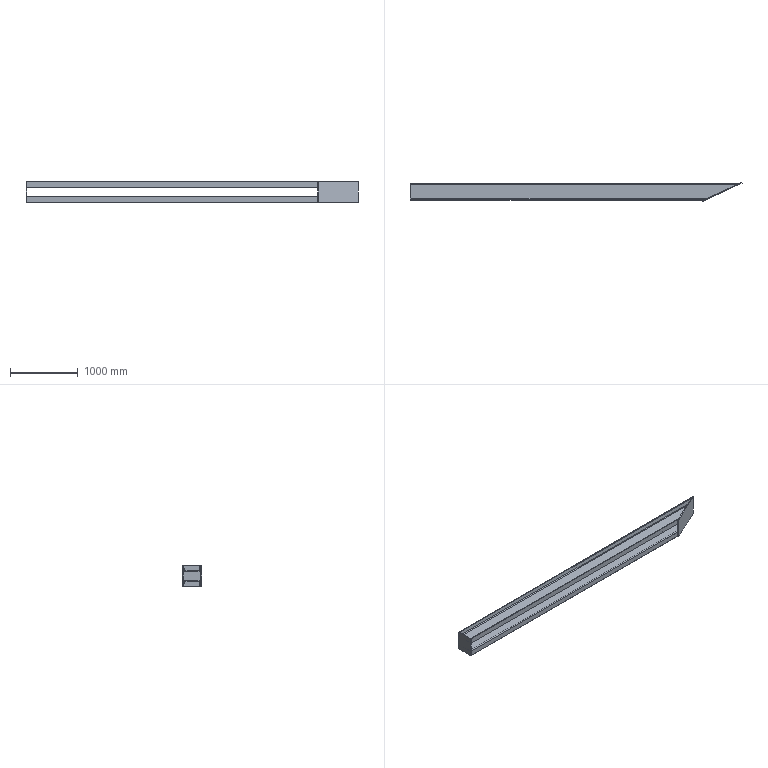Part | STEP file | Lower channel steel_Default<As machined> | 4 solids | 40 faces | box 4891 x 283.464 x 300 mm | volume 35069262 mm3 | plane 32 | cylinder 8 | commonest cylinder face diameters 12 x4 24 x4